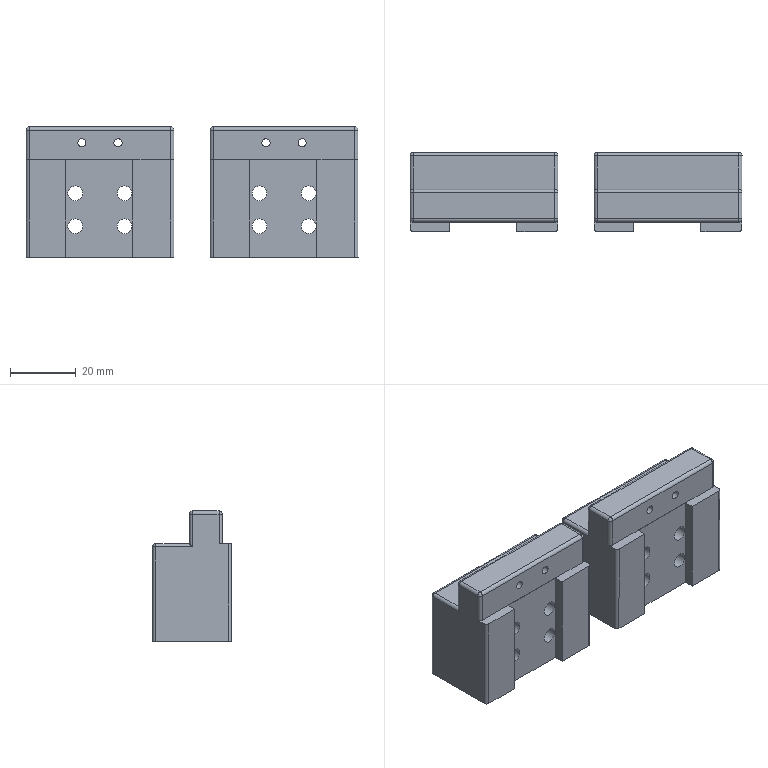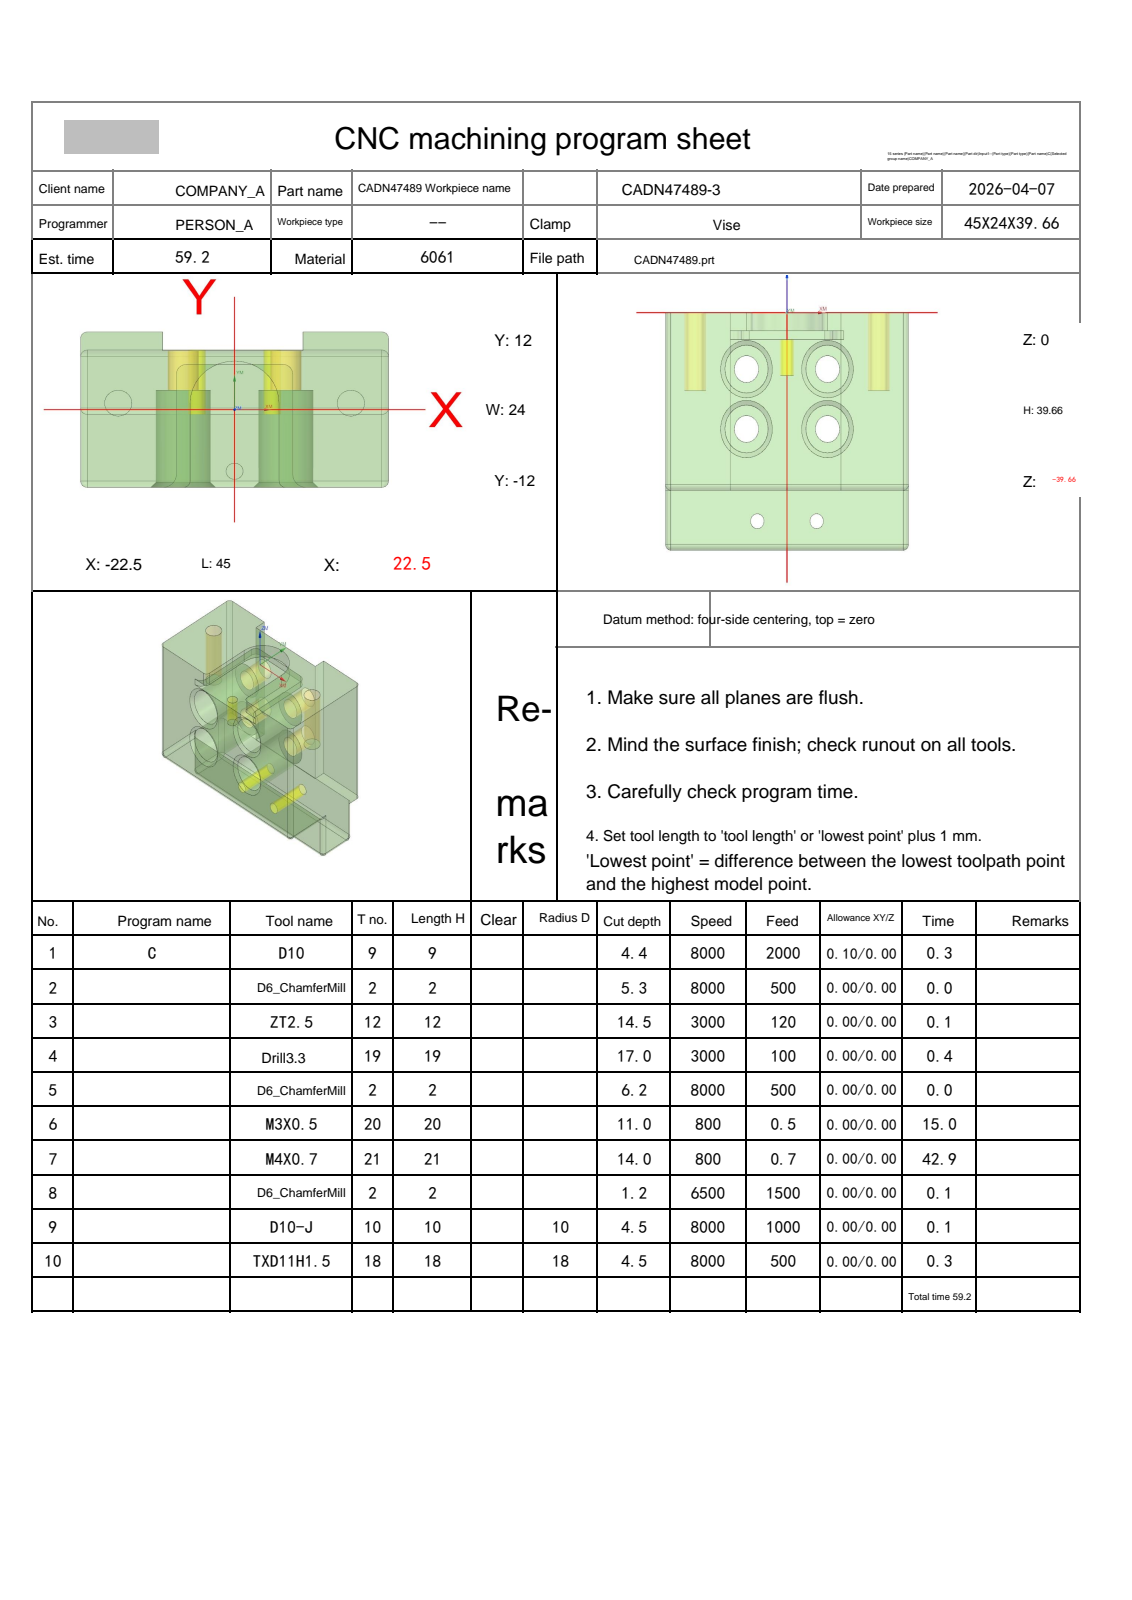NC program | NX | posted by the shop | part box 101.001 x 24.001 x 39.667 mm
Whole program:
%
O0001
(Machine time: 114.21 MIN)
(===Total Tool:8===)
(T9=D10     D=10.  R=0.   D9  H09 Z=-4.4  )
(T2=D6_ChamferMill   D=6.   R=0.   D-  H02 Z=-6.25 )
(T12=ZT2.5  D=2.5  DR_a=118 D-  H12 Z=-14.5 )
(T19=Drill 3.3  D=3.3  DR_a=118 D-  H19 Z=-17.  )
(T20=M3X0.5 D=2.5  DR_a=180 D-  H20 Z=-11.  )
(T21=M4X0.7 D=3.3  DR_a=180 D-  H21 Z=-14.  )
(T10=D10-J  D=10.  R=0.   D10 H10 Z=-4.5  )
(T18=TXD11H1.5 D=11.  CR=0.  D18 H18 Z=-4.5  )
G80 G90 G17 G49 G40
G91 G28 Z0
M01
N1 T09 M06
(D10  D=10. R=0. H=09 ce=0.10 di=0.10)
G00 G90 G54 X8.853 Y-20.1 M03 S8000
G43 H09 Z10.1
M08
Z.95
G01 Z-.55 F2000.
Y-17.662
X5.951 Y-16.9
G02 X1.4 Y-11. I1.549 J5.9
G01 Y1.
G03 X1.072 Y1.9 I-1.4 J0.0
G01 X-1.072
G03 X-1.4 Y1. I1.072 J-.9
G01 Y-11.
G02 X-5.951 Y-16.9 I-6.1 J0.0
G01 X-8.852 Y-17.662
Y-20.1
Z.95
G00 X8.853
Z.4
G01 Z-1.1
Y-17.662
X5.951 Y-16.9
G02 X1.4 Y-11. I1.549 J5.9
G01 Y1.
G03 X1.072 Y1.9 I-1.4 J0.0
G01 X-1.072
G03 X-1.4 Y1. I1.072 J-.9
G01 Y-11.
G02 X-5.951 Y-16.9 I-6.1 J0.0
G01 X-8.852 Y-17.662
Y-20.1
Z.4
G00 X8.853
Z-.15
G01 Z-1.65
Y-17.662
X5.951 Y-16.9
G02 X1.4 Y-11. I1.549 J5.9
G01 Y1.
G03 X1.072 Y1.9 I-1.4 J0.0
G01 X-1.072
G03 X-1.4 Y1. I1.072 J-.9
G01 Y-11.
G02 X-5.951 Y-16.9 I-6.1 J0.0
G01 X-8.852 Y-17.662
Y-20.1
Z-.15
G00 X8.853
Z-.7
G01 Z-2.2
Y-17.662
X5.951 Y-16.9
G02 X1.4 Y-11. I1.549 J5.9
G01 Y1.
G03 X1.072 Y1.9 I-1.4 J0.0
G01 X-1.072
G03 X-1.4 Y1. I1.072 J-.9
G01 Y-11.
G02 X-5.951 Y-16.9 I-6.1 J0.0
G01 X-8.852 Y-17.662
Y-20.1
Z-.7
G00 X8.853
Z-1.25
G01 Z-2.75
Y-17.662
X5.951 Y-16.9
G02 X1.4 Y-11. I1.549 J5.9
G01 Y1.
G03 X1.072 Y1.9 I-1.4 J0.0
G01 X-1.072
G03 X-1.4 Y1. I1.072 J-.9
G01 Y-11.
G02 X-5.951 Y-16.9 I-6.1 J0.0
G01 X-8.852 Y-17.662
Y-20.1
Z-1.25
G00 X8.853
Z-1.8
G01 Z-3.3
Y-17.662
X5.951 Y-16.9
G02 X1.4 Y-11. I1.549 J5.9
G01 Y1.
G03 X1.072 Y1.9 I-1.4 J0.0
G01 X-1.072
G03 X-1.4 Y1. I1.072 J-.9
G01 Y-11.
G02 X-5.951 Y-16.9 I-6.1 J0.0
G01 X-8.852 Y-17.662
Y-20.1
Z-1.8
G00 X8.853
Z-2.35
G01 Z-3.85
Y-17.662
X5.951 Y-16.9
G02 X1.4 Y-11. I1.549 J5.9
G01 Y1.
G03 X1.072 Y1.9 I-1.4 J0.0
G01 X-1.072
G03 X-1.4 Y1. I1.072 J-.9
G01 Y-11.
G02 X-5.951 Y-16.9 I-6.1 J0.0
G01 X-8.852 Y-17.662
Y-20.1
Z-2.35
G00 X8.853
Z-2.9
G01 Z-4.4
Y-17.662
X5.951 Y-16.9
G02 X1.4 Y-11. I1.549 J5.9
G01 Y1.
G03 X1.072 Y1.9 I-1.4 J0.0
G01 X-1.072
G03 X-1.4 Y1. I1.072 J-.9
G01 Y-11.
G02 X-5.951 Y-16.9 I-6.1 J0.0
G01 X-8.852 Y-17.662
Y-20.1
Z-2.9
G00 Z10.1
G00 G90 X8.915 Y-18.8 M03 S8000
Z5.1
Z-2.
G01 Z-3. F1000.
G41 D09
Y-18.6
G03 X7.432 Y-17.1 I-1.5 J0.0
G02 X1.4 Y-11. I.068 J6.1
G01 Y-10.988
Y1.007
G03 X1.29 Y1.543 I-1.4 J-.007
X0.0 Y2.4 I-1.29 J-.543
X-1.4 Y1. I0.0 J-1.4
G01 Y.992
Y-11.018
G02 X-7.48 Y-17.1 I-6.1 J.018
G03 X-8.975 Y-18.6 I.005 J-1.5
G01 G40 Y-18.8
Z-2.
G00 Z5.1
G91 G28 Z0.0
M05
M09
G91 G28 Z0.0
M01
N2 T02 M06
(D6_ChamferMill  D=6. R=0. H=02 ce=0.00 di=0.00)
G00 G90 G54 X-17. Y1. M03 S8000
G43 H02 Z20.
M08
G98 G81 X-17. Y1. Z-.8 R1. F500.
X0.0 Y-9.5 Z-5.3 R-3.5
X17. Y1. Z-.8 R1.
G80
G00 Z20.
G91 G28 Z0.0
M05
M09
G91 G28 Z0.0
M01
N3 T12 M06
(ZT2.5 D=2.5 DR_a=118 H=12)
G00 G90 G54 X0.0 Y-9.5 M03 S3000
G43 H12 Z20.
M08
G98 G83 X0.0 Y-9.5 Z-14.5 R-3.5 F120. Q2.
G80
G00 Z20.
G91 G28 Z0.0
M05
M09
G91 G28 Z0.0
M01
N4 T19 M06
(Drill 3.3 D=3.3 DR_a=118 H=19)
G00 G90 G54 X-17. Y1. M03 S3000
G43 H19 Z20.
M08
G98 G83 X-17. Y1. Z-17. R1. F100. Q2.
X17.
G80
G00 Z20.
G91 G28 Z0.0
M05
M09
G91 G28 Z0.0
M01
N5 T02 M06
(D6_ChamferMill  D=6. R=0. H=02 ce=0.00 di=0.00)
G00 G90 G54 X0.0 Y-9.5 M03 S8000
G43 H02 Z20.
M08
G98 G81 X0.0 Y-9.5 Z-6.25 R-1.5 F500.
G80
G00 Z20.
G00 G90 X-17. Y1. M03 S8000
Z20.
G98 G81 X-17. Y1. Z-2.2 R3. F500.
X17.
G80
G00 Z20.
G91 G28 Z0.0
M05
M09
G91 G28 Z0.0
M01
N6 T20 M06
(M3X0.5 D=2.5 DR_a=180 H=20)
G00 G90 G54 X0.0 Y-9.5 M03 S800
G43 H20 Z20.
M08
G95
G98 G84 X0.0 Y-9.5 Z-11. R-3.5 F.5 Q2.
G80
G94
G00 Z20.
G91 G28 Z0.0
M05
M09
G91 G28 Z0.0
M01
N7 T21 M06
(M4X0.7 D=3.3 DR_a=180 H=21)
G00 G90 G54 X-17. Y1. M03 S800
G43 H21 Z20.
M08
G95
G98 G84 X-17. Y1. Z-14. R1. F.7 Q4.
X17.
G80
G94
G00 Z20.
G91 G28 Z0.0
M05
M09
G91 G28 Z0.0
M01
N8 T02 M06
(D6_ChamferMill  D=6. R=0. H=02 ce=0.00 di=0.00)
G00 G90 G54 X23.727 Y.386 M03 S6500
G43 H02 Z20.
M08
Z.172
G01 Z-1.2 F1500.
G03 X23.527 Y.1 I1.532 J-1.286
G01 X23.497 Y.054
X23.5 Y0.0
Y-11.
G02 X21.5 Y-13. I-2. J0.0
G01 X7.5
G02 X5.5 Y-11. I0.0 J2.
G01 Y1.
G03 X0.0 Y6.5 I-5.5 J0.0
X-5.5 Y1. I0.0 J-5.5
G01 Y-11.
G02 X-7.5 Y-13. I-2. J0.0
G01 X-21.5
G02 X-23.5 Y-11. I0.0 J2.
G01 Y11.
G02 X-21.5 Y13. I2. J0.0
G01 X-10.5
G02 X-9.5 Y12. I0.0 J-1.
G01 Y10.1
X9.
Y12.
G02 X10. Y13. I1. J0.0
G01 X21.5
G02 X23.5 Y11. I0.0 J-2.
G01 Y0.0
X23.497 Y-.054
X23.527 Y-.1
G03 X23.727 Y-.386 I1.732 J1.
G01 Z.172
G00 Z10.
X-17.494 Y1.419
Z.406
G01 Z-1.2
G03 X-17.641 Y1.103 I1.732 J-1.
G01 X-17.662 Y1.053
X-17.65 Y1.
G03 X-17. Y.35 I.65 J0.0
X-16.35 Y1. I0.0 J.65
X-17. Y1.65 I-.65 J0.0
X-17.65 Y1. I0.0 J-.65
G01 X-17.662 Y.947
X-17.641 Y.897
G03 X-17.494 Y.581 I1.879 J.684
G01 Z.403
G00 Z10.
X16.506 Y1.419
Z.404
G01 Z-1.2
G03 X16.359 Y1.103 I1.732 J-1.
G01 X16.338 Y1.053
X16.35 Y1.
G03 X17. Y.35 I.65 J0.0
X17.65 Y1. I0.0 J.65
X17. Y1.65 I-.65 J0.0
X16.35 Y1. I0.0 J-.65
G01 X16.338 Y.947
X16.359 Y.897
G03 X16.506 Y.581 I1.879 J.684
G01 Z.406
G00 Z20.
G91 G28 Z0.0
M05
M09
G91 G28 Z0.0
M01
N9 T10 M06
(D10-J  D=10. R=0. H=10 ce=0.00 di=0.00)
G00 G90 G54 X9.247 Y-19.2 M03 S8000
G43 H10 Z10.
M08
Z-3.5
G01 Z-4.5 F1000.
G41 D10
Y-19.
Y-18.996
G03 X7.31 Y-16.997 I-2. J0.0
G02 X1.5 Y-11. I.19 J5.997
G01 Y1.
G03 X1.118 Y2. I-1.5 J0.0
G01 X-1.118
G03 X-1.5 Y1. I1.118 J-1.
G01 Y-11.
G02 X-7.31 Y-16.997 I-6. J0.0
G03 X-9.247 Y-18.996 I.063 J-1.999
G01 Y-19.
G40 Y-19.2
Z-3.5
G00 Z10.
G00 G90 X8.92 Y-18.7 M03 S8000
Z5.
Z-2.
G01 Z-3. F1000.
G41 D10
Y-18.5
G03 X7.436 Y-17. I-1.5 J0.0
G02 X1.5 Y-11. I.064 J6.
G01 Y-10.99
Y1.001
G03 X1.149 Y1.964 I-1.5 J-.001
X0.0 Y2.5 I-1.149 J-.964
X-1.5 Y1. I0.0 J-1.5
G01 Y.991
Y-11.017
G02 X-7.48 Y-17. I-6. J.017
G03 X-8.976 Y-18.5 I.005 J-1.5
G01 G40 Y-18.7
Z-2.
G00 Z5.
G91 G28 Z0.0
M05
M09
G91 G28 Z0.0
M01
N10 T18 M06
(TXD11H1.5 D=11. CR=0. H=18 ce=0.80 di=0.00)
G00 G90 G54 X12.7 Y-20.7 M03 S8000
G43 H18 Z20.
M08
Z-3.5
G01 Z-4.5 F500.
G41 D10
Y-20.5
G03 X10.5 Y-18.3 I-2.2 J0.0
G02 X2.2 Y-10. I0.0 J8.3
G01 Y.7
X-2.2
Y-10.
G02 X-10.5 Y-18.3 I-8.3 J0.0
G03 X-12.7 Y-20.5 I0.0 J-2.2
G01 G40 Y-20.7
Z-3.5
G00 Z20.
G00 G90 X12.7 Y-19.9 M03 S8000
Z20.
Z-3.5
G01 Z-4.5 F500.
G41 D10
Y-19.7
G03 X10.5 Y-17.5 I-2.2 J0.0
G02 X3. Y-10. I0.0 J7.5
G01 Y1.5
X-3.
Y-10.
G02 X-10.5 Y-17.5 I-7.5 J0.0
G03 X-12.7 Y-19.7 I0.0 J-2.2
G01 G40 Y-19.9
Z-3.5
G00 Z20.
M05
M09
G91 G28 Z0.0
G91 G28 Y0.0
M30
%